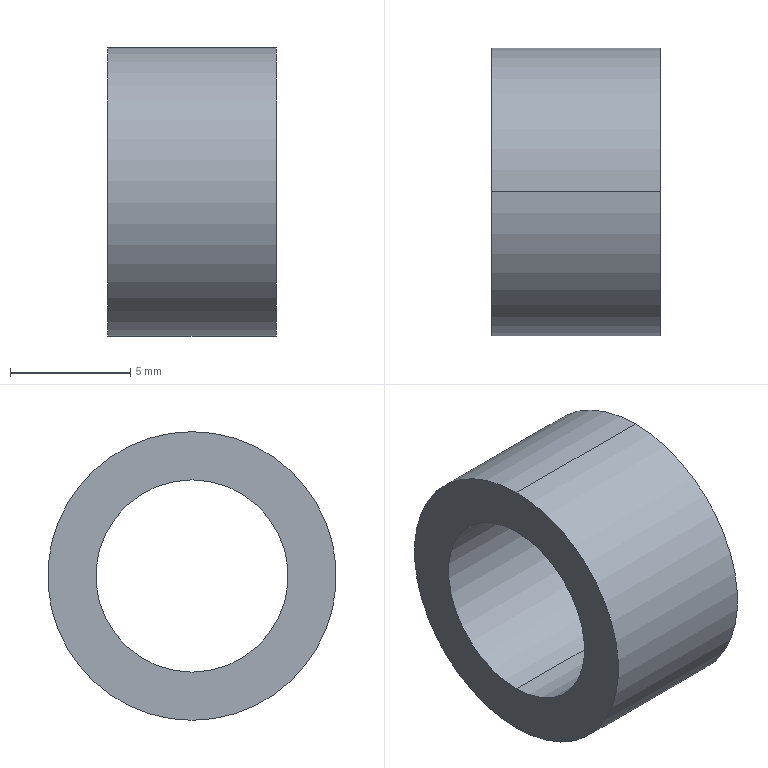Part | SolidWorks | features BaseBody 1 | 1 solid | 6 faces | box 7 x 12 x 12 mm | volume 439.823 mm3 | cylinder 4 | plane 2 | commonest cylinder face diameters 8 x2 12 x2
STEP:
#1=CARTESIAN_POINT('',(-3.5,0.,-6.));
#2=VERTEX_POINT('',#1);
#3=CARTESIAN_POINT('',(-3.5,0.,6.));
#4=VERTEX_POINT('',#3);
#5=CARTESIAN_POINT('',(-3.5,0.,0.));
#6=DIRECTION('',(1.,0.,0.));
#7=DIRECTION('',(0.,0.,-1.));
#8=AXIS2_PLACEMENT_3D('',#5,#6,#7);
#9=CIRCLE('',#8,6.);
#10=EDGE_CURVE('',#2,#4,#9,.T.);
#11=ORIENTED_EDGE('',*,*,#10,.T.);
#12=CARTESIAN_POINT('',(3.5,0.,6.));
#13=VERTEX_POINT('',#12);
#14=CARTESIAN_POINT('',(-3.5,0.,6.));
#15=DIRECTION('',(1.,0.,0.));
#16=VECTOR('',#15,1000.);
#17=LINE('',#14,#16);
#18=EDGE_CURVE('',#4,#13,#17,.T.);
#19=ORIENTED_EDGE('',*,*,#18,.T.);
#20=CARTESIAN_POINT('',(3.5,0.,-6.));
#21=VERTEX_POINT('',#20);
#22=CARTESIAN_POINT('',(3.5,0.,0.));
#23=DIRECTION('',(-1.,0.,0.));
#24=DIRECTION('',(0.,0.,-1.));
#25=AXIS2_PLACEMENT_3D('',#22,#23,#24);
#26=CIRCLE('',#25,6.);
#27=EDGE_CURVE('',#13,#21,#26,.T.);
#28=ORIENTED_EDGE('',*,*,#27,.T.);
#29=CARTESIAN_POINT('',(-3.5,0.,-6.));
#30=DIRECTION('',(1.,0.,0.));
#31=VECTOR('',#30,1000.);
#32=LINE('',#29,#31);
#33=EDGE_CURVE('',#2,#21,#32,.T.);
#34=ORIENTED_EDGE('',*,*,#33,.F.);
#35=EDGE_LOOP('',(#11,#19,#28,#34));
#36=FACE_OUTER_BOUND('',#35,.T.);
#37=CARTESIAN_POINT('',(-3.5,0.,0.));
#38=DIRECTION('',(1.,0.,0.));
#39=DIRECTION('',(0.,0.,-1.));
#40=AXIS2_PLACEMENT_3D('',#37,#38,#39);
#41=CYLINDRICAL_SURFACE('',#40,6.);
#42=ADVANCED_FACE('',(#36),#41,.T.);
#43=CARTESIAN_POINT('',(-3.5,0.,-4.));
#44=VERTEX_POINT('',#43);
#45=CARTESIAN_POINT('',(-3.5,0.,4.));
#46=VERTEX_POINT('',#45);
#47=CARTESIAN_POINT('',(-3.5,0.,0.));
#48=DIRECTION('',(-1.,0.,0.));
#49=DIRECTION('',(0.,0.,-1.));
#50=AXIS2_PLACEMENT_3D('',#47,#48,#49);
#51=CIRCLE('',#50,4.);
#52=EDGE_CURVE('',#44,#46,#51,.T.);
#53=ORIENTED_EDGE('',*,*,#52,.T.);
#54=CARTESIAN_POINT('',(3.5,0.,4.));
#55=VERTEX_POINT('',#54);
#56=CARTESIAN_POINT('',(-4.5,0.,4.));
#57=DIRECTION('',(1.,0.,0.));
#58=VECTOR('',#57,1000.);
#59=LINE('',#56,#58);
#60=EDGE_CURVE('',#46,#55,#59,.T.);
#61=ORIENTED_EDGE('',*,*,#60,.T.);
#62=CARTESIAN_POINT('',(3.5,0.,-4.));
#63=VERTEX_POINT('',#62);
#64=CARTESIAN_POINT('',(3.5,0.,0.));
#65=DIRECTION('',(-1.,0.,0.));
#66=DIRECTION('',(0.,0.,-1.));
#67=AXIS2_PLACEMENT_3D('',#64,#65,#66);
#68=CIRCLE('',#67,4.);
#69=EDGE_CURVE('',#63,#55,#68,.T.);
#70=ORIENTED_EDGE('',*,*,#69,.F.);
#71=CARTESIAN_POINT('',(-4.5,0.,-4.));
#72=DIRECTION('',(1.,0.,0.));
#73=VECTOR('',#72,1000.);
#74=LINE('',#71,#73);
#75=EDGE_CURVE('',#44,#63,#74,.T.);
#76=ORIENTED_EDGE('',*,*,#75,.F.);
#77=EDGE_LOOP('',(#53,#61,#70,#76));
#78=FACE_OUTER_BOUND('',#77,.T.);
#79=CARTESIAN_POINT('',(-4.5,0.,0.));
#80=DIRECTION('',(1.,0.,0.));
#81=DIRECTION('',(0.,0.,-1.));
#82=AXIS2_PLACEMENT_3D('',#79,#80,#81);
#83=CYLINDRICAL_SURFACE('',#82,4.);
#84=ADVANCED_FACE('',(#78),#83,.F.);
#85=ORIENTED_EDGE('',*,*,#18,.F.);
#86=CARTESIAN_POINT('',(-3.5,0.,0.));
#87=DIRECTION('',(1.,0.,0.));
#88=DIRECTION('',(0.,0.,-1.));
#89=AXIS2_PLACEMENT_3D('',#86,#87,#88);
#90=CIRCLE('',#89,6.);
#91=EDGE_CURVE('',#4,#2,#90,.T.);
#92=ORIENTED_EDGE('',*,*,#91,.T.);
#93=ORIENTED_EDGE('',*,*,#33,.T.);
#94=CARTESIAN_POINT('',(3.5,0.,0.));
#95=DIRECTION('',(-1.,0.,0.));
#96=DIRECTION('',(0.,0.,-1.));
#97=AXIS2_PLACEMENT_3D('',#94,#95,#96);
#98=CIRCLE('',#97,6.);
#99=EDGE_CURVE('',#21,#13,#98,.T.);
#100=ORIENTED_EDGE('',*,*,#99,.T.);
#101=EDGE_LOOP('',(#85,#92,#93,#100));
#102=FACE_OUTER_BOUND('',#101,.T.);
#103=CARTESIAN_POINT('',(-3.5,0.,0.));
#104=DIRECTION('',(1.,0.,0.));
#105=DIRECTION('',(0.,0.,-1.));
#106=AXIS2_PLACEMENT_3D('',#103,#104,#105);
#107=CYLINDRICAL_SURFACE('',#106,6.);
#108=ADVANCED_FACE('',(#102),#107,.T.);
#109=ORIENTED_EDGE('',*,*,#52,.F.);
#110=CARTESIAN_POINT('',(-3.5,0.,0.));
#111=DIRECTION('',(-1.,0.,0.));
#112=DIRECTION('',(0.,0.,-1.));
#113=AXIS2_PLACEMENT_3D('',#110,#111,#112);
#114=CIRCLE('',#113,4.);
#115=EDGE_CURVE('',#46,#44,#114,.T.);
#116=ORIENTED_EDGE('',*,*,#115,.F.);
#117=EDGE_LOOP('',(#109,#116));
#118=FACE_BOUND('',#117,.T.);
#119=ORIENTED_EDGE('',*,*,#10,.F.);
#120=ORIENTED_EDGE('',*,*,#91,.F.);
#121=EDGE_LOOP('',(#119,#120));
#122=FACE_OUTER_BOUND('',#121,.T.);
#123=CARTESIAN_POINT('',(-3.5,0.,0.));
#124=DIRECTION('',(1.,0.,0.));
#125=DIRECTION('',(0.,0.,-1.));
#126=AXIS2_PLACEMENT_3D('',#123,#124,#125);
#127=PLANE('',#126);
#128=ADVANCED_FACE('',(#118,#122),#127,.F.);
#129=ORIENTED_EDGE('',*,*,#69,.T.);
#130=CARTESIAN_POINT('',(3.5,0.,0.));
#131=DIRECTION('',(-1.,0.,0.));
#132=DIRECTION('',(0.,0.,-1.));
#133=AXIS2_PLACEMENT_3D('',#130,#131,#132);
#134=CIRCLE('',#133,4.);
#135=EDGE_CURVE('',#55,#63,#134,.T.);
#136=ORIENTED_EDGE('',*,*,#135,.T.);
#137=EDGE_LOOP('',(#129,#136));
#138=FACE_BOUND('',#137,.T.);
#139=ORIENTED_EDGE('',*,*,#99,.F.);
#140=ORIENTED_EDGE('',*,*,#27,.F.);
#141=EDGE_LOOP('',(#139,#140));
#142=FACE_OUTER_BOUND('',#141,.T.);
#143=CARTESIAN_POINT('',(3.5,0.,0.));
#144=DIRECTION('',(1.,0.,0.));
#145=DIRECTION('',(0.,0.,-1.));
#146=AXIS2_PLACEMENT_3D('',#143,#144,#145);
#147=PLANE('',#146);
#148=ADVANCED_FACE('',(#138,#142),#147,.T.);
#149=ORIENTED_EDGE('',*,*,#60,.F.);
#150=ORIENTED_EDGE('',*,*,#115,.T.);
#151=ORIENTED_EDGE('',*,*,#75,.T.);
#152=ORIENTED_EDGE('',*,*,#135,.F.);
#153=EDGE_LOOP('',(#149,#150,#151,#152));
#154=FACE_OUTER_BOUND('',#153,.T.);
#155=CARTESIAN_POINT('',(-4.5,0.,0.));
#156=DIRECTION('',(1.,0.,0.));
#157=DIRECTION('',(0.,0.,-1.));
#158=AXIS2_PLACEMENT_3D('',#155,#156,#157);
#159=CYLINDRICAL_SURFACE('',#158,4.);
#160=ADVANCED_FACE('',(#154),#159,.F.);
#161=CLOSED_SHELL('',(#42,#84,#108,#128,#148,#160));
#162=MANIFOLD_SOLID_BREP('',#161);
#163=CARTESIAN_POINT('',(0.,0.,0.));
#164=DIRECTION('',(0.,0.,1.));
#165=DIRECTION('',(1.,0.,0.));
#166=AXIS2_PLACEMENT_3D('',#163,#164,#165);
#167=(LENGTH_UNIT()NAMED_UNIT(*)SI_UNIT(.MILLI.,.METRE.));
#168=UNCERTAINTY_MEASURE_WITH_UNIT(LENGTH_MEASURE(0.00001),#167,'','');
#169=(NAMED_UNIT(*)PLANE_ANGLE_UNIT()SI_UNIT($,.RADIAN.));
#170=(NAMED_UNIT(*)SI_UNIT($,.STERADIAN.)SOLID_ANGLE_UNIT());
#171=(GEOMETRIC_REPRESENTATION_CONTEXT(3)GLOBAL_UNCERTAINTY_ASSIGNED_CONTEXT((#168))GLOBAL_UNIT_ASSIGNED_CONTEXT((#167,#169,#170))REPRESENTATION_CONTEXT('',''));
#172=ADVANCED_BREP_SHAPE_REPRESENTATION('',(#162,#166),#171);